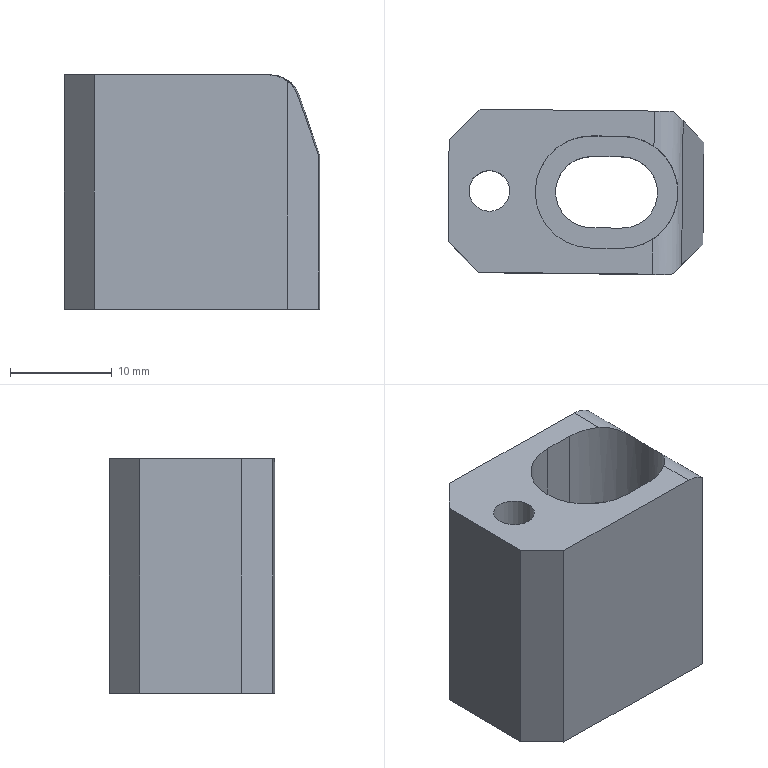Part | NX | features solid 2 | 1 solid | 22 faces | box 25.103 x 16.198 x 23 mm | volume 6372 mm3 | plane 16 | cylinder 6 | commonest cylinder face diameters 7 x2 11 x2 4.001 x1 6 x1
STEP:
#1=CARTESIAN_POINT('',(1618.85,304.866,17.4));
#2=VERTEX_POINT('',#1);
#3=CARTESIAN_POINT('',(1635.95,304.687,17.4));
#4=VERTEX_POINT('',#3);
#5=CARTESIAN_POINT('',(1630.849,304.74,17.4));
#6=DIRECTION('',(0.9999,-0.01047,0.));
#7=VECTOR('',#6,1000.);
#8=LINE('',#5,#7);
#9=EDGE_CURVE('',#2,#4,#8,.T.);
#10=ORIENTED_EDGE('',*,*,#9,.T.);
#11=CARTESIAN_POINT('',(1635.986,308.144,17.4));
#12=VERTEX_POINT('',#11);
#13=CARTESIAN_POINT('',(1636.034,312.686,17.4));
#14=DIRECTION('',(-0.01047,-0.9999,0.));
#15=VECTOR('',#14,1000.);
#16=LINE('',#13,#15);
#17=EDGE_CURVE('',#12,#4,#16,.T.);
#18=ORIENTED_EDGE('',*,*,#17,.F.);
#19=CARTESIAN_POINT('',(1632.875,307.219,17.4));
#20=VERTEX_POINT('',#19);
#21=CARTESIAN_POINT('',(1632.933,312.719,17.4));
#22=DIRECTION('',(0.,0.,1.));
#23=DIRECTION('',(-0.1736,-0.9848,0.));
#24=AXIS2_PLACEMENT_3D('',#21,#22,#23);
#25=CIRCLE('',#24,5.5);
#26=EDGE_CURVE('',#20,#12,#25,.T.);
#27=ORIENTED_EDGE('',*,*,#26,.F.);
#28=CARTESIAN_POINT('',(1629.875,307.25,17.4));
#29=VERTEX_POINT('',#28);
#30=CARTESIAN_POINT('',(1630.875,307.24,17.4));
#31=DIRECTION('',(0.9999,-0.01047,0.));
#32=VECTOR('',#31,1000.);
#33=LINE('',#30,#32);
#34=EDGE_CURVE('',#29,#20,#33,.T.);
#35=ORIENTED_EDGE('',*,*,#34,.F.);
#36=CARTESIAN_POINT('',(1629.99,318.25,17.4));
#37=VERTEX_POINT('',#36);
#38=CARTESIAN_POINT('',(1629.933,312.75,17.4));
#39=DIRECTION('',(0.,0.,1.));
#40=DIRECTION('',(-0.1736,-0.9848,0.));
#41=AXIS2_PLACEMENT_3D('',#38,#39,#40);
#42=CIRCLE('',#41,5.5);
#43=EDGE_CURVE('',#37,#29,#42,.T.);
#44=ORIENTED_EDGE('',*,*,#43,.F.);
#45=CARTESIAN_POINT('',(1632.99,318.218,17.4));
#46=VERTEX_POINT('',#45);
#47=CARTESIAN_POINT('',(1630.99,318.239,17.4));
#48=DIRECTION('',(-0.9999,0.01047,0.));
#49=VECTOR('',#48,1000.);
#50=LINE('',#47,#49);
#51=EDGE_CURVE('',#46,#37,#50,.T.);
#52=ORIENTED_EDGE('',*,*,#51,.F.);
#53=CARTESIAN_POINT('',(1636.081,317.228,17.4));
#54=VERTEX_POINT('',#53);
#55=CARTESIAN_POINT('',(1632.933,312.719,17.4));
#56=DIRECTION('',(0.,0.,1.));
#57=DIRECTION('',(-0.1736,-0.9848,0.));
#58=AXIS2_PLACEMENT_3D('',#55,#56,#57);
#59=CIRCLE('',#58,5.5);
#60=EDGE_CURVE('',#54,#46,#59,.T.);
#61=ORIENTED_EDGE('',*,*,#60,.F.);
#62=CARTESIAN_POINT('',(1636.118,320.686,17.4));
#63=VERTEX_POINT('',#62);
#64=CARTESIAN_POINT('',(1636.034,312.686,17.4));
#65=DIRECTION('',(-0.01047,-0.9999,0.));
#66=VECTOR('',#65,1000.);
#67=LINE('',#64,#66);
#68=EDGE_CURVE('',#63,#54,#67,.T.);
#69=ORIENTED_EDGE('',*,*,#68,.F.);
#70=CARTESIAN_POINT('',(1619.017,320.865,17.4));
#71=VERTEX_POINT('',#70);
#72=CARTESIAN_POINT('',(1631.017,320.739,17.4));
#73=DIRECTION('',(-0.9999,0.01047,0.));
#74=VECTOR('',#73,1000.);
#75=LINE('',#72,#74);
#76=EDGE_CURVE('',#63,#71,#75,.T.);
#77=ORIENTED_EDGE('',*,*,#76,.T.);
#78=CARTESIAN_POINT('',(1615.986,317.896,17.4));
#79=VERTEX_POINT('',#78);
#80=CARTESIAN_POINT('',(1620.533,322.349,17.4));
#81=DIRECTION('',(0.7145,0.6997,0.));
#82=VECTOR('',#81,1000.);
#83=LINE('',#80,#82);
#84=EDGE_CURVE('',#79,#71,#83,.T.);
#85=ORIENTED_EDGE('',*,*,#84,.F.);
#86=CARTESIAN_POINT('',(1615.881,307.897,17.4));
#87=VERTEX_POINT('',#86);
#88=CARTESIAN_POINT('',(1615.934,312.897,17.4));
#89=DIRECTION('',(-0.01047,-0.9999,0.));
#90=VECTOR('',#89,1000.);
#91=LINE('',#88,#90);
#92=EDGE_CURVE('',#79,#87,#91,.T.);
#93=ORIENTED_EDGE('',*,*,#92,.T.);
#94=CARTESIAN_POINT('',(1620.334,303.35,17.4));
#95=DIRECTION('',(-0.6997,0.7145,0.));
#96=VECTOR('',#95,1000.);
#97=LINE('',#94,#96);
#98=EDGE_CURVE('',#2,#87,#97,.T.);
#99=ORIENTED_EDGE('',*,*,#98,.F.);
#100=EDGE_LOOP('',(#10,#18,#27,#35,#44,#52,#61,#69,#77,#85,#93,#99));
#101=FACE_BOUND('',#100,.T.);
#102=CARTESIAN_POINT('',(1619.49,314.806,17.4));
#103=VERTEX_POINT('',#102);
#104=CARTESIAN_POINT('',(1619.933,312.855,17.4));
#105=DIRECTION('',(0.,0.,1.));
#106=DIRECTION('',(-0.2215,0.9751,0.));
#107=AXIS2_PLACEMENT_3D('',#104,#105,#106);
#108=CIRCLE('',#107,2.001);
#109=EDGE_CURVE('',#103,#103,#108,.T.);
#110=ORIENTED_EDGE('',*,*,#109,.F.);
#111=EDGE_LOOP('',(#110));
#112=FACE_BOUND('',#111,.T.);
#113=CARTESIAN_POINT('',(1630.933,312.74,17.4));
#114=DIRECTION('',(0.,0.,1.));
#115=DIRECTION('',(0.184,0.9829,0.));
#116=AXIS2_PLACEMENT_3D('',#113,#114,#115);
#117=PLANE('',#116);
#118=ADVANCED_FACE('',(#101,#112),#117,.T.);
#119=CARTESIAN_POINT('',(1620.417,314.796,-5.6));
#120=VERTEX_POINT('',#119);
#121=CARTESIAN_POINT('',(1619.933,312.855,-5.6));
#122=DIRECTION('',(0.,0.,1.));
#123=DIRECTION('',(0.2419,0.9703,0.));
#124=AXIS2_PLACEMENT_3D('',#121,#122,#123);
#125=CIRCLE('',#124,2.001);
#126=EDGE_CURVE('',#120,#120,#125,.T.);
#127=ORIENTED_EDGE('',*,*,#126,.T.);
#128=EDGE_LOOP('',(#127));
#129=FACE_BOUND('',#128,.T.);
#130=CARTESIAN_POINT('',(1637.849,304.667,-5.6));
#131=VERTEX_POINT('',#130);
#132=CARTESIAN_POINT('',(1618.85,304.866,-5.6));
#133=VERTEX_POINT('',#132);
#134=CARTESIAN_POINT('',(1630.849,304.74,-5.6));
#135=DIRECTION('',(-0.9999,0.01047,0.));
#136=VECTOR('',#135,1000.);
#137=LINE('',#134,#136);
#138=EDGE_CURVE('',#131,#133,#137,.T.);
#139=ORIENTED_EDGE('',*,*,#138,.T.);
#140=CARTESIAN_POINT('',(1615.881,307.897,-5.6));
#141=VERTEX_POINT('',#140);
#142=CARTESIAN_POINT('',(1619.839,303.855,-5.6));
#143=DIRECTION('',(0.6997,-0.7145,0.));
#144=VECTOR('',#143,1000.);
#145=LINE('',#142,#144);
#146=EDGE_CURVE('',#141,#133,#145,.T.);
#147=ORIENTED_EDGE('',*,*,#146,.F.);
#148=CARTESIAN_POINT('',(1615.986,317.896,-5.6));
#149=VERTEX_POINT('',#148);
#150=CARTESIAN_POINT('',(1615.934,312.897,-5.6));
#151=DIRECTION('',(0.01047,0.9999,0.));
#152=VECTOR('',#151,1000.);
#153=LINE('',#150,#152);
#154=EDGE_CURVE('',#141,#149,#153,.T.);
#155=ORIENTED_EDGE('',*,*,#154,.T.);
#156=CARTESIAN_POINT('',(1619.017,320.865,-5.6));
#157=VERTEX_POINT('',#156);
#158=CARTESIAN_POINT('',(1620.028,321.854,-5.6));
#159=DIRECTION('',(-0.7145,-0.6997,0.));
#160=VECTOR('',#159,1000.);
#161=LINE('',#158,#160);
#162=EDGE_CURVE('',#157,#149,#161,.T.);
#163=ORIENTED_EDGE('',*,*,#162,.F.);
#164=CARTESIAN_POINT('',(1638.016,320.666,-5.6));
#165=VERTEX_POINT('',#164);
#166=CARTESIAN_POINT('',(1631.017,320.739,-5.6));
#167=DIRECTION('',(0.9999,-0.01047,0.));
#168=VECTOR('',#167,1000.);
#169=LINE('',#166,#168);
#170=EDGE_CURVE('',#157,#165,#169,.T.);
#171=ORIENTED_EDGE('',*,*,#170,.T.);
#172=CARTESIAN_POINT('',(1640.985,317.635,-5.6));
#173=VERTEX_POINT('',#172);
#174=CARTESIAN_POINT('',(1638.511,320.161,-5.6));
#175=DIRECTION('',(-0.6997,0.7145,0.));
#176=VECTOR('',#175,1000.);
#177=LINE('',#174,#176);
#178=EDGE_CURVE('',#173,#165,#177,.T.);
#179=ORIENTED_EDGE('',*,*,#178,.F.);
#180=CARTESIAN_POINT('',(1640.88,307.635,-5.6));
#181=VERTEX_POINT('',#180);
#182=CARTESIAN_POINT('',(1640.932,312.635,-5.6));
#183=DIRECTION('',(-0.01047,-0.9999,0.));
#184=VECTOR('',#183,1000.);
#185=LINE('',#182,#184);
#186=EDGE_CURVE('',#173,#181,#185,.T.);
#187=ORIENTED_EDGE('',*,*,#186,.T.);
#188=CARTESIAN_POINT('',(1638.354,305.161,-5.6));
#189=DIRECTION('',(0.7145,0.6997,0.));
#190=VECTOR('',#189,1000.);
#191=LINE('',#188,#190);
#192=EDGE_CURVE('',#131,#181,#191,.T.);
#193=ORIENTED_EDGE('',*,*,#192,.F.);
#194=EDGE_LOOP('',(#139,#147,#155,#163,#171,#179,#187,#193));
#195=FACE_BOUND('',#194,.T.);
#196=CARTESIAN_POINT('',(1632.969,316.218,-5.6));
#197=VERTEX_POINT('',#196);
#198=CARTESIAN_POINT('',(1632.896,309.219,-5.6));
#199=VERTEX_POINT('',#198);
#200=CARTESIAN_POINT('',(1632.933,312.719,-5.6));
#201=DIRECTION('',(0.,0.,-1.));
#202=DIRECTION('',(0.2419,0.9703,0.));
#203=AXIS2_PLACEMENT_3D('',#200,#201,#202);
#204=CIRCLE('',#203,3.5);
#205=EDGE_CURVE('',#197,#199,#204,.T.);
#206=ORIENTED_EDGE('',*,*,#205,.F.);
#207=CARTESIAN_POINT('',(1629.969,316.25,-5.6));
#208=VERTEX_POINT('',#207);
#209=CARTESIAN_POINT('',(1630.969,316.239,-5.6));
#210=DIRECTION('',(0.9999,-0.01047,0.));
#211=VECTOR('',#210,1000.);
#212=LINE('',#209,#211);
#213=EDGE_CURVE('',#208,#197,#212,.T.);
#214=ORIENTED_EDGE('',*,*,#213,.F.);
#215=CARTESIAN_POINT('',(1629.896,309.25,-5.6));
#216=VERTEX_POINT('',#215);
#217=CARTESIAN_POINT('',(1629.933,312.75,-5.6));
#218=DIRECTION('',(0.,0.,-1.));
#219=DIRECTION('',(0.2419,0.9703,0.));
#220=AXIS2_PLACEMENT_3D('',#217,#218,#219);
#221=CIRCLE('',#220,3.5);
#222=EDGE_CURVE('',#216,#208,#221,.T.);
#223=ORIENTED_EDGE('',*,*,#222,.F.);
#224=CARTESIAN_POINT('',(1630.896,309.24,-5.6));
#225=DIRECTION('',(-0.9999,0.01047,0.));
#226=VECTOR('',#225,1000.);
#227=LINE('',#224,#226);
#228=EDGE_CURVE('',#199,#216,#227,.T.);
#229=ORIENTED_EDGE('',*,*,#228,.F.);
#230=EDGE_LOOP('',(#206,#214,#223,#229));
#231=FACE_BOUND('',#230,.T.);
#232=CARTESIAN_POINT('',(1630.933,312.74,-5.6));
#233=DIRECTION('',(0.,0.,-1.));
#234=DIRECTION('',(-0.184,-0.9829,0.));
#235=AXIS2_PLACEMENT_3D('',#232,#233,#234);
#236=PLANE('',#235);
#237=ADVANCED_FACE('',(#129,#195,#231),#236,.T.);
#238=ORIENTED_EDGE('',*,*,#186,.F.);
#239=CARTESIAN_POINT('',(1640.985,317.635,9.4));
#240=VERTEX_POINT('',#239);
#241=CARTESIAN_POINT('',(1640.985,317.635,2.4));
#242=DIRECTION('',(0.,0.,-1.));
#243=VECTOR('',#242,1000.);
#244=LINE('',#241,#243);
#245=EDGE_CURVE('',#240,#173,#244,.T.);
#246=ORIENTED_EDGE('',*,*,#245,.F.);
#247=CARTESIAN_POINT('',(1640.88,307.635,9.4));
#248=VERTEX_POINT('',#247);
#249=CARTESIAN_POINT('',(1640.932,312.635,9.4));
#250=DIRECTION('',(0.01047,0.9999,0.));
#251=VECTOR('',#250,1000.);
#252=LINE('',#249,#251);
#253=EDGE_CURVE('',#248,#240,#252,.T.);
#254=ORIENTED_EDGE('',*,*,#253,.F.);
#255=CARTESIAN_POINT('',(1640.88,307.635,2.4));
#256=DIRECTION('',(0.,0.,1.));
#257=VECTOR('',#256,1000.);
#258=LINE('',#255,#257);
#259=EDGE_CURVE('',#181,#248,#258,.T.);
#260=ORIENTED_EDGE('',*,*,#259,.F.);
#261=EDGE_LOOP('',(#238,#246,#254,#260));
#262=FACE_BOUND('',#261,.T.);
#263=CARTESIAN_POINT('',(1640.932,312.635,2.4));
#264=DIRECTION('',(0.9999,-0.01047,0.));
#265=DIRECTION('',(0.01047,0.9999,0.));
#266=AXIS2_PLACEMENT_3D('',#263,#264,#265);
#267=PLANE('',#266);
#268=ADVANCED_FACE('',(#262),#267,.T.);
#269=ORIENTED_EDGE('',*,*,#170,.F.);
#270=CARTESIAN_POINT('',(1619.017,320.865,2.4));
#271=DIRECTION('',(0.,0.,-1.));
#272=VECTOR('',#271,1000.);
#273=LINE('',#270,#272);
#274=EDGE_CURVE('',#71,#157,#273,.T.);
#275=ORIENTED_EDGE('',*,*,#274,.F.);
#276=ORIENTED_EDGE('',*,*,#76,.F.);
#277=CARTESIAN_POINT('',(1638.016,320.666,16.723));
#278=VERTEX_POINT('',#277);
#279=CARTESIAN_POINT('',(1636.118,320.686,14.4));
#280=DIRECTION('',(-0.01047,-0.9999,0.));
#281=DIRECTION('',(0.9999,-0.01047,0.));
#282=AXIS2_PLACEMENT_3D('',#279,#280,#281);
#283=CIRCLE('',#282,3.);
#284=EDGE_CURVE('',#278,#63,#283,.T.);
#285=ORIENTED_EDGE('',*,*,#284,.F.);
#286=CARTESIAN_POINT('',(1638.016,320.666,2.4));
#287=DIRECTION('',(0.,0.,1.));
#288=VECTOR('',#287,1000.);
#289=LINE('',#286,#288);
#290=EDGE_CURVE('',#165,#278,#289,.T.);
#291=ORIENTED_EDGE('',*,*,#290,.F.);
#292=EDGE_LOOP('',(#269,#275,#276,#285,#291));
#293=FACE_BOUND('',#292,.T.);
#294=CARTESIAN_POINT('',(1631.017,320.739,2.4));
#295=DIRECTION('',(0.01047,0.9999,0.));
#296=DIRECTION('',(-0.9999,0.01047,0.));
#297=AXIS2_PLACEMENT_3D('',#294,#295,#296);
#298=PLANE('',#297);
#299=ADVANCED_FACE('',(#293),#298,.T.);
#300=ORIENTED_EDGE('',*,*,#92,.F.);
#301=CARTESIAN_POINT('',(1615.986,317.896,2.4));
#302=DIRECTION('',(0.,0.,1.));
#303=VECTOR('',#302,1000.);
#304=LINE('',#301,#303);
#305=EDGE_CURVE('',#149,#79,#304,.T.);
#306=ORIENTED_EDGE('',*,*,#305,.F.);
#307=ORIENTED_EDGE('',*,*,#154,.F.);
#308=CARTESIAN_POINT('',(1615.881,307.897,2.4));
#309=DIRECTION('',(0.,0.,-1.));
#310=VECTOR('',#309,1000.);
#311=LINE('',#308,#310);
#312=EDGE_CURVE('',#87,#141,#311,.T.);
#313=ORIENTED_EDGE('',*,*,#312,.F.);
#314=EDGE_LOOP('',(#300,#306,#307,#313));
#315=FACE_BOUND('',#314,.T.);
#316=CARTESIAN_POINT('',(1615.934,312.897,2.4));
#317=DIRECTION('',(-0.9999,0.01047,0.));
#318=DIRECTION('',(-0.01047,-0.9999,0.));
#319=AXIS2_PLACEMENT_3D('',#316,#317,#318);
#320=PLANE('',#319);
#321=ADVANCED_FACE('',(#315),#320,.T.);
#322=CARTESIAN_POINT('',(1637.849,304.667,16.723));
#323=VERTEX_POINT('',#322);
#324=CARTESIAN_POINT('',(1635.95,304.687,14.4));
#325=DIRECTION('',(0.01047,0.9999,0.));
#326=DIRECTION('',(-0.9999,0.01047,0.));
#327=AXIS2_PLACEMENT_3D('',#324,#325,#326);
#328=CIRCLE('',#327,3.);
#329=EDGE_CURVE('',#4,#323,#328,.T.);
#330=ORIENTED_EDGE('',*,*,#329,.F.);
#331=ORIENTED_EDGE('',*,*,#9,.F.);
#332=CARTESIAN_POINT('',(1618.85,304.866,2.4));
#333=DIRECTION('',(0.,0.,1.));
#334=VECTOR('',#333,1000.);
#335=LINE('',#332,#334);
#336=EDGE_CURVE('',#133,#2,#335,.T.);
#337=ORIENTED_EDGE('',*,*,#336,.F.);
#338=ORIENTED_EDGE('',*,*,#138,.F.);
#339=CARTESIAN_POINT('',(1637.849,304.667,2.4));
#340=DIRECTION('',(0.,0.,-1.));
#341=VECTOR('',#340,1000.);
#342=LINE('',#339,#341);
#343=EDGE_CURVE('',#323,#131,#342,.T.);
#344=ORIENTED_EDGE('',*,*,#343,.F.);
#345=EDGE_LOOP('',(#330,#331,#337,#338,#344));
#346=FACE_BOUND('',#345,.T.);
#347=CARTESIAN_POINT('',(1630.849,304.74,2.4));
#348=DIRECTION('',(-0.01047,-0.9999,0.));
#349=DIRECTION('',(0.9999,-0.01047,0.));
#350=AXIS2_PLACEMENT_3D('',#347,#348,#349);
#351=PLANE('',#350);
#352=ADVANCED_FACE('',(#346),#351,.T.);
#353=CARTESIAN_POINT('',(1629.896,309.25,8.4));
#354=VERTEX_POINT('',#353);
#355=CARTESIAN_POINT('',(1629.969,316.25,8.4));
#356=VERTEX_POINT('',#355);
#357=CARTESIAN_POINT('',(1629.933,312.75,8.4));
#358=DIRECTION('',(0.,0.,-1.));
#359=DIRECTION('',(0.1736,0.9848,0.));
#360=AXIS2_PLACEMENT_3D('',#357,#358,#359);
#361=CIRCLE('',#360,3.5);
#362=EDGE_CURVE('',#354,#356,#361,.T.);
#363=ORIENTED_EDGE('',*,*,#362,.T.);
#364=CARTESIAN_POINT('',(1632.969,316.218,8.4));
#365=VERTEX_POINT('',#364);
#366=CARTESIAN_POINT('',(1630.068,316.249,8.4));
#367=DIRECTION('',(-0.9999,0.01047,0.));
#368=VECTOR('',#367,1000.);
#369=LINE('',#366,#368);
#370=EDGE_CURVE('',#365,#356,#369,.T.);
#371=ORIENTED_EDGE('',*,*,#370,.F.);
#372=CARTESIAN_POINT('',(1632.896,309.219,8.4));
#373=VERTEX_POINT('',#372);
#374=CARTESIAN_POINT('',(1632.933,312.719,8.4));
#375=DIRECTION('',(0.,0.,1.));
#376=DIRECTION('',(0.1736,0.9848,0.));
#377=AXIS2_PLACEMENT_3D('',#374,#375,#376);
#378=CIRCLE('',#377,3.5);
#379=EDGE_CURVE('',#373,#365,#378,.T.);
#380=ORIENTED_EDGE('',*,*,#379,.F.);
#381=CARTESIAN_POINT('',(1629.995,309.249,8.4));
#382=DIRECTION('',(0.9999,-0.01047,0.));
#383=VECTOR('',#382,1000.);
#384=LINE('',#381,#383);
#385=EDGE_CURVE('',#354,#373,#384,.T.);
#386=ORIENTED_EDGE('',*,*,#385,.F.);
#387=EDGE_LOOP('',(#363,#371,#380,#386));
#388=FACE_BOUND('',#387,.T.);
#389=CARTESIAN_POINT('',(1632.875,307.219,8.4));
#390=VERTEX_POINT('',#389);
#391=CARTESIAN_POINT('',(1632.99,318.218,8.4));
#392=VERTEX_POINT('',#391);
#393=CARTESIAN_POINT('',(1632.933,312.719,8.4));
#394=DIRECTION('',(0.,0.,1.));
#395=DIRECTION('',(0.1736,0.9848,0.));
#396=AXIS2_PLACEMENT_3D('',#393,#394,#395);
#397=CIRCLE('',#396,5.5);
#398=EDGE_CURVE('',#390,#392,#397,.T.);
#399=ORIENTED_EDGE('',*,*,#398,.T.);
#400=CARTESIAN_POINT('',(1629.99,318.25,8.4));
#401=VERTEX_POINT('',#400);
#402=CARTESIAN_POINT('',(1628.99,318.26,8.4));
#403=DIRECTION('',(0.9999,-0.01047,0.));
#404=VECTOR('',#403,1000.);
#405=LINE('',#402,#404);
#406=EDGE_CURVE('',#401,#392,#405,.T.);
#407=ORIENTED_EDGE('',*,*,#406,.F.);
#408=CARTESIAN_POINT('',(1629.875,307.25,8.4));
#409=VERTEX_POINT('',#408);
#410=CARTESIAN_POINT('',(1629.933,312.75,8.4));
#411=DIRECTION('',(0.,0.,-1.));
#412=DIRECTION('',(0.1736,0.9848,0.));
#413=AXIS2_PLACEMENT_3D('',#410,#411,#412);
#414=CIRCLE('',#413,5.5);
#415=EDGE_CURVE('',#409,#401,#414,.T.);
#416=ORIENTED_EDGE('',*,*,#415,.F.);
#417=CARTESIAN_POINT('',(1628.875,307.261,8.4));
#418=DIRECTION('',(-0.9999,0.01047,0.));
#419=VECTOR('',#418,1000.);
#420=LINE('',#417,#419);
#421=EDGE_CURVE('',#390,#409,#420,.T.);
#422=ORIENTED_EDGE('',*,*,#421,.F.);
#423=EDGE_LOOP('',(#399,#407,#416,#422));
#424=FACE_BOUND('',#423,.T.);
#425=CARTESIAN_POINT('',(1628.933,312.761,8.4));
#426=DIRECTION('',(0.,0.,-1.));
#427=DIRECTION('',(-0.1736,-0.9848,0.));
#428=AXIS2_PLACEMENT_3D('',#425,#426,#427);
#429=PLANE('',#428);
#430=ADVANCED_FACE('',(#388,#424),#429,.F.);
#431=ORIENTED_EDGE('',*,*,#222,.T.);
#432=CARTESIAN_POINT('',(1629.969,316.25,5.4));
#433=DIRECTION('',(0.,0.,-1.));
#434=VECTOR('',#433,1000.);
#435=LINE('',#432,#434);
#436=EDGE_CURVE('',#356,#208,#435,.T.);
#437=ORIENTED_EDGE('',*,*,#436,.F.);
#438=ORIENTED_EDGE('',*,*,#362,.F.);
#439=CARTESIAN_POINT('',(1629.896,309.25,5.4));
#440=DIRECTION('',(0.,0.,1.));
#441=VECTOR('',#440,1000.);
#442=LINE('',#439,#441);
#443=EDGE_CURVE('',#216,#354,#442,.T.);
#444=ORIENTED_EDGE('',*,*,#443,.F.);
#445=EDGE_LOOP('',(#431,#437,#438,#444));
#446=FACE_BOUND('',#445,.T.);
#447=CARTESIAN_POINT('',(1629.933,312.75,22.4));
#448=DIRECTION('',(0.,0.,-1.));
#449=DIRECTION('',(0.1736,0.9848,0.));
#450=AXIS2_PLACEMENT_3D('',#447,#448,#449);
#451=CYLINDRICAL_SURFACE('',#450,3.5);
#452=ADVANCED_FACE('',(#446),#451,.F.);
#453=ORIENTED_EDGE('',*,*,#415,.T.);
#454=CARTESIAN_POINT('',(1629.99,318.25,12.9));
#455=DIRECTION('',(0.,0.,-1.));
#456=VECTOR('',#455,1000.);
#457=LINE('',#454,#456);
#458=EDGE_CURVE('',#37,#401,#457,.T.);
#459=ORIENTED_EDGE('',*,*,#458,.F.);
#460=ORIENTED_EDGE('',*,*,#43,.T.);
#461=CARTESIAN_POINT('',(1629.875,307.25,12.9));
#462=DIRECTION('',(0.,0.,1.));
#463=VECTOR('',#462,1000.);
#464=LINE('',#461,#463);
#465=EDGE_CURVE('',#409,#29,#464,.T.);
#466=ORIENTED_EDGE('',*,*,#465,.F.);
#467=EDGE_LOOP('',(#453,#459,#460,#466));
#468=FACE_BOUND('',#467,.T.);
#469=CARTESIAN_POINT('',(1629.933,312.75,22.4));
#470=DIRECTION('',(0.,0.,-1.));
#471=DIRECTION('',(0.1736,0.9848,0.));
#472=AXIS2_PLACEMENT_3D('',#469,#470,#471);
#473=CYLINDRICAL_SURFACE('',#472,5.5);
#474=ADVANCED_FACE('',(#468),#473,.F.);
#475=ORIENTED_EDGE('',*,*,#379,.T.);
#476=CARTESIAN_POINT('',(1632.969,316.218,5.4));
#477=DIRECTION('',(0.,0.,1.));
#478=VECTOR('',#477,1000.);
#479=LINE('',#476,#478);
#480=EDGE_CURVE('',#197,#365,#479,.T.);
#481=ORIENTED_EDGE('',*,*,#480,.F.);
#482=ORIENTED_EDGE('',*,*,#205,.T.);
#483=CARTESIAN_POINT('',(1632.896,309.219,5.4));
#484=DIRECTION('',(0.,0.,-1.));
#485=VECTOR('',#484,1000.);
#486=LINE('',#483,#485);
#487=EDGE_CURVE('',#373,#199,#486,.T.);
#488=ORIENTED_EDGE('',*,*,#487,.F.);
#489=EDGE_LOOP('',(#475,#481,#482,#488));
#490=FACE_BOUND('',#489,.T.);
#491=CARTESIAN_POINT('',(1632.933,312.719,22.4));
#492=DIRECTION('',(0.,0.,-1.));
#493=DIRECTION('',(0.1736,0.9848,0.));
#494=AXIS2_PLACEMENT_3D('',#491,#492,#493);
#495=CYLINDRICAL_SURFACE('',#494,3.5);
#496=ADVANCED_FACE('',(#490),#495,.F.);
#497=ORIENTED_EDGE('',*,*,#26,.T.);
#498=CARTESIAN_POINT('',(1636.081,317.228,17.4));
#499=CARTESIAN_POINT('',(1636.844,316.696,17.4));
#500=CARTESIAN_POINT('',(1638.006,315.341,16.852));
#501=CARTESIAN_POINT('',(1638.659,312.657,15.876));
#502=CARTESIAN_POINT('',(1637.95,309.991,16.852));
#503=CARTESIAN_POINT('',(1636.759,308.66,17.4));
#504=CARTESIAN_POINT('',(1635.986,308.144,17.4));
#505=B_SPLINE_CURVE_WITH_KNOTS('',3,(#498,#499,#500,#501,#502,#503,#504),.UNSPECIFIED.,.F.,.F.,(4,1,1,1,4),(0.,0.002735,0.00547,0.008205,0.01094),.UNSPECIFIED.);
#506=EDGE_CURVE('',#54,#12,#505,.T.);
#507=ORIENTED_EDGE('',*,*,#506,.F.);
#508=ORIENTED_EDGE('',*,*,#60,.T.);
#509=CARTESIAN_POINT('',(1632.99,318.218,12.9));
#510=DIRECTION('',(0.,0.,1.));
#511=VECTOR('',#510,1000.);
#512=LINE('',#509,#511);
#513=EDGE_CURVE('',#392,#46,#512,.T.);
#514=ORIENTED_EDGE('',*,*,#513,.F.);
#515=ORIENTED_EDGE('',*,*,#398,.F.);
#516=CARTESIAN_POINT('',(1632.875,307.219,12.9));
#517=DIRECTION('',(0.,0.,-1.));
#518=VECTOR('',#517,1000.);
#519=LINE('',#516,#518);
#520=EDGE_CURVE('',#20,#390,#519,.T.);
#521=ORIENTED_EDGE('',*,*,#520,.F.);
#522=EDGE_LOOP('',(#497,#507,#508,#514,#515,#521));
#523=FACE_BOUND('',#522,.T.);
#524=CARTESIAN_POINT('',(1632.933,312.719,22.4));
#525=DIRECTION('',(0.,0.,-1.));
#526=DIRECTION('',(0.1736,0.9848,0.));
#527=AXIS2_PLACEMENT_3D('',#524,#525,#526);
#528=CYLINDRICAL_SURFACE('',#527,5.5);
#529=ADVANCED_FACE('',(#523),#528,.F.);
#530=ORIENTED_EDGE('',*,*,#253,.T.);
#531=CARTESIAN_POINT('',(1638.943,319.719,15.378));
#532=VERTEX_POINT('',#531);
#533=CARTESIAN_POINT('',(1642.344,316.246,5.418));
#534=DIRECTION('',(0.3068,-0.3133,-0.8987));
#535=VECTOR('',#534,1000.);
#536=LINE('',#533,#535);
#537=EDGE_CURVE('',#532,#240,#536,.T.);
#538=ORIENTED_EDGE('',*,*,#537,.F.);
#539=CARTESIAN_POINT('',(1638.796,305.594,15.378));
#540=VERTEX_POINT('',#539);
#541=CARTESIAN_POINT('',(1638.87,312.656,15.378));
#542=DIRECTION('',(0.01047,0.9999,0.));
#543=VECTOR('',#542,1000.);
#544=LINE('',#541,#543);
#545=EDGE_CURVE('',#540,#532,#544,.T.);
#546=ORIENTED_EDGE('',*,*,#545,.F.);
#547=CARTESIAN_POINT('',(1642.851,309.565,3.746));
#548=DIRECTION('',(-0.3133,-0.3068,0.8987));
#549=VECTOR('',#548,1000.);
#550=LINE('',#547,#549);
#551=EDGE_CURVE('',#248,#540,#550,.T.);
#552=ORIENTED_EDGE('',*,*,#551,.F.);
#553=EDGE_LOOP('',(#530,#538,#546,#552));
#554=FACE_BOUND('',#553,.T.);
#555=CARTESIAN_POINT('',(1640.932,312.635,9.4));
#556=DIRECTION('',(-0.9453,0.009899,-0.3262));
#557=DIRECTION('',(-0.01047,-0.9999,0.));
#558=AXIS2_PLACEMENT_3D('',#555,#556,#557);
#559=PLANE('',#558);
#560=ADVANCED_FACE('',(#554),#559,.F.);
#561=ORIENTED_EDGE('',*,*,#545,.T.);
#562=CARTESIAN_POINT('',(1636.137,322.584,14.4));
#563=DIRECTION('',(0.7145,0.6997,0.));
#564=DIRECTION('',(-0.6997,0.7145,0.));
#565=AXIS2_PLACEMENT_3D('',#562,#563,#564);
#566=ELLIPSE('',#565,4.243,3.);
#567=EDGE_CURVE('',#278,#532,#566,.T.);
#568=ORIENTED_EDGE('',*,*,#567,.F.);
#569=ORIENTED_EDGE('',*,*,#284,.T.);
#570=ORIENTED_EDGE('',*,*,#68,.T.);
#571=ORIENTED_EDGE('',*,*,#506,.T.);
#572=ORIENTED_EDGE('',*,*,#17,.T.);
#573=ORIENTED_EDGE('',*,*,#329,.T.);
#574=CARTESIAN_POINT('',(1635.93,302.788,14.4));
#575=DIRECTION('',(0.6997,-0.7145,0.));
#576=DIRECTION('',(0.7145,0.6997,0.));
#577=AXIS2_PLACEMENT_3D('',#574,#575,#576);
#578=ELLIPSE('',#577,4.243,3.);
#579=EDGE_CURVE('',#540,#323,#578,.T.);
#580=ORIENTED_EDGE('',*,*,#579,.F.);
#581=EDGE_LOOP('',(#561,#568,#569,#570,#571,#572,#573,#580));
#582=FACE_BOUND('',#581,.T.);
#583=CARTESIAN_POINT('',(1636.034,312.686,14.4));
#584=DIRECTION('',(0.01047,0.9999,0.));
#585=DIRECTION('',(-0.9999,0.01047,0.));
#586=AXIS2_PLACEMENT_3D('',#583,#584,#585);
#587=CYLINDRICAL_SURFACE('',#586,3.);
#588=ADVANCED_FACE('',(#582),#587,.T.);
#589=ORIENTED_EDGE('',*,*,#51,.T.);
#590=ORIENTED_EDGE('',*,*,#458,.T.);
#591=ORIENTED_EDGE('',*,*,#406,.T.);
#592=ORIENTED_EDGE('',*,*,#513,.T.);
#593=EDGE_LOOP('',(#589,#590,#591,#592));
#594=FACE_BOUND('',#593,.T.);
#595=CARTESIAN_POINT('',(1630.026,318.249,22.4));
#596=DIRECTION('',(0.01047,0.9999,0.));
#597=DIRECTION('',(0.,0.,1.));
#598=AXIS2_PLACEMENT_3D('',#595,#596,#597);
#599=PLANE('',#598);
#600=ADVANCED_FACE('',(#594),#599,.F.);
#601=ORIENTED_EDGE('',*,*,#370,.T.);
#602=ORIENTED_EDGE('',*,*,#436,.T.);
#603=ORIENTED_EDGE('',*,*,#213,.T.);
#604=ORIENTED_EDGE('',*,*,#480,.T.);
#605=EDGE_LOOP('',(#601,#602,#603,#604));
#606=FACE_BOUND('',#605,.T.);
#607=CARTESIAN_POINT('',(1630.068,316.249,22.4));
#608=DIRECTION('',(0.01047,0.9999,0.));
#609=DIRECTION('',(0.,0.,1.));
#610=AXIS2_PLACEMENT_3D('',#607,#608,#609);
#611=PLANE('',#610);
#612=ADVANCED_FACE('',(#606),#611,.F.);
#613=ORIENTED_EDGE('',*,*,#228,.T.);
#614=ORIENTED_EDGE('',*,*,#443,.T.);
#615=ORIENTED_EDGE('',*,*,#385,.T.);
#616=ORIENTED_EDGE('',*,*,#487,.T.);
#617=EDGE_LOOP('',(#613,#614,#615,#616));
#618=FACE_BOUND('',#617,.T.);
#619=CARTESIAN_POINT('',(1629.995,309.249,22.4));
#620=DIRECTION('',(-0.01047,-0.9999,0.));
#621=DIRECTION('',(0.,0.,-1.));
#622=AXIS2_PLACEMENT_3D('',#619,#620,#621);
#623=PLANE('',#622);
#624=ADVANCED_FACE('',(#618),#623,.F.);
#625=ORIENTED_EDGE('',*,*,#421,.T.);
#626=ORIENTED_EDGE('',*,*,#465,.T.);
#627=ORIENTED_EDGE('',*,*,#34,.T.);
#628=ORIENTED_EDGE('',*,*,#520,.T.);
#629=EDGE_LOOP('',(#625,#626,#627,#628));
#630=FACE_BOUND('',#629,.T.);
#631=CARTESIAN_POINT('',(1629.911,307.25,22.4));
#632=DIRECTION('',(-0.01047,-0.9999,0.));
#633=DIRECTION('',(0.,0.,-1.));
#634=AXIS2_PLACEMENT_3D('',#631,#632,#633);
#635=PLANE('',#634);
#636=ADVANCED_FACE('',(#630),#635,.F.);
#637=ORIENTED_EDGE('',*,*,#146,.T.);
#638=ORIENTED_EDGE('',*,*,#336,.T.);
#639=ORIENTED_EDGE('',*,*,#98,.T.);
#640=ORIENTED_EDGE('',*,*,#312,.T.);
#641=EDGE_LOOP('',(#637,#638,#639,#640));
#642=FACE_BOUND('',#641,.T.);
#643=CARTESIAN_POINT('',(1618.85,304.866,2.4));
#644=DIRECTION('',(0.7145,0.6997,0.));
#645=DIRECTION('',(0.,0.,-1.));
#646=AXIS2_PLACEMENT_3D('',#643,#644,#645);
#647=PLANE('',#646);
#648=ADVANCED_FACE('',(#642),#647,.F.);
#649=ORIENTED_EDGE('',*,*,#162,.T.);
#650=ORIENTED_EDGE('',*,*,#305,.T.);
#651=ORIENTED_EDGE('',*,*,#84,.T.);
#652=ORIENTED_EDGE('',*,*,#274,.T.);
#653=EDGE_LOOP('',(#649,#650,#651,#652));
#654=FACE_BOUND('',#653,.T.);
#655=CARTESIAN_POINT('',(1615.986,317.896,2.4));
#656=DIRECTION('',(0.6997,-0.7145,0.));
#657=DIRECTION('',(0.,0.,-1.));
#658=AXIS2_PLACEMENT_3D('',#655,#656,#657);
#659=PLANE('',#658);
#660=ADVANCED_FACE('',(#654),#659,.F.);
#661=ORIENTED_EDGE('',*,*,#178,.T.);
#662=ORIENTED_EDGE('',*,*,#290,.T.);
#663=ORIENTED_EDGE('',*,*,#567,.T.);
#664=ORIENTED_EDGE('',*,*,#537,.T.);
#665=ORIENTED_EDGE('',*,*,#245,.T.);
#666=EDGE_LOOP('',(#661,#662,#663,#664,#665));
#667=FACE_BOUND('',#666,.T.);
#668=CARTESIAN_POINT('',(1638.016,320.666,2.4));
#669=DIRECTION('',(-0.7145,-0.6997,0.));
#670=DIRECTION('',(0.,0.,-1.));
#671=AXIS2_PLACEMENT_3D('',#668,#669,#670);
#672=PLANE('',#671);
#673=ADVANCED_FACE('',(#667),#672,.F.);
#674=ORIENTED_EDGE('',*,*,#192,.T.);
#675=ORIENTED_EDGE('',*,*,#259,.T.);
#676=ORIENTED_EDGE('',*,*,#551,.T.);
#677=ORIENTED_EDGE('',*,*,#579,.T.);
#678=ORIENTED_EDGE('',*,*,#343,.T.);
#679=EDGE_LOOP('',(#674,#675,#676,#677,#678));
#680=FACE_BOUND('',#679,.T.);
#681=CARTESIAN_POINT('',(1640.88,307.635,2.4));
#682=DIRECTION('',(-0.6997,0.7145,0.));
#683=DIRECTION('',(0.,0.,-1.));
#684=AXIS2_PLACEMENT_3D('',#681,#682,#683);
#685=PLANE('',#684);
#686=ADVANCED_FACE('',(#680),#685,.F.);
#687=ORIENTED_EDGE('',*,*,#109,.T.);
#688=EDGE_LOOP('',(#687));
#689=FACE_BOUND('',#688,.T.);
#690=ORIENTED_EDGE('',*,*,#126,.F.);
#691=EDGE_LOOP('',(#690));
#692=FACE_BOUND('',#691,.T.);
#693=CARTESIAN_POINT('',(1619.933,312.855,17.4));
#694=DIRECTION('',(0.,0.,-1.));
#695=DIRECTION('',(-0.2215,0.9751,0.));
#696=AXIS2_PLACEMENT_3D('',#693,#694,#695);
#697=CYLINDRICAL_SURFACE('',#696,2.001);
#698=ADVANCED_FACE('',(#689,#692),#697,.F.);
#699=CLOSED_SHELL('',(#118,#237,#268,#299,#321,#352,#430,#452,#474,#496,#529,#560,#588,#600,#612,#624,#636,#648,#660,#673,#686,#698));
#700=MANIFOLD_SOLID_BREP('',#699);
#701=(LENGTH_UNIT()NAMED_UNIT(*)SI_UNIT(.MILLI.,.METRE.));
#702=UNCERTAINTY_MEASURE_WITH_UNIT(LENGTH_MEASURE(0.0508),#701,'','');
#703=(NAMED_UNIT(*)PLANE_ANGLE_UNIT()SI_UNIT($,.RADIAN.));
#704=(NAMED_UNIT(*)SI_UNIT($,.STERADIAN.)SOLID_ANGLE_UNIT());
#705=(GEOMETRIC_REPRESENTATION_CONTEXT(3)GLOBAL_UNCERTAINTY_ASSIGNED_CONTEXT((#702))GLOBAL_UNIT_ASSIGNED_CONTEXT((#701,#703,#704))REPRESENTATION_CONTEXT('',''));
#706=ADVANCED_BREP_SHAPE_REPRESENTATION('',(#700),#705);